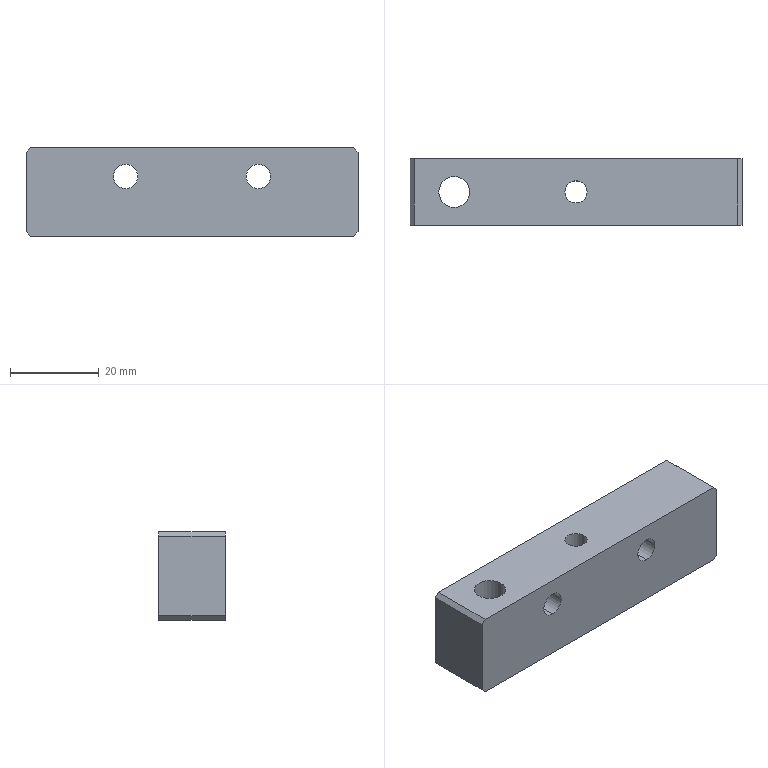Part | STEP file | PN_0111 buffer mounting seat | 1 solid | 24 faces | box 75 x 15 x 20 mm | volume 19970 mm3 | cylinder 12 | plane 12 | commonest cylinder face diameters 5.5 x4 10 x4 5 x2 7 x2